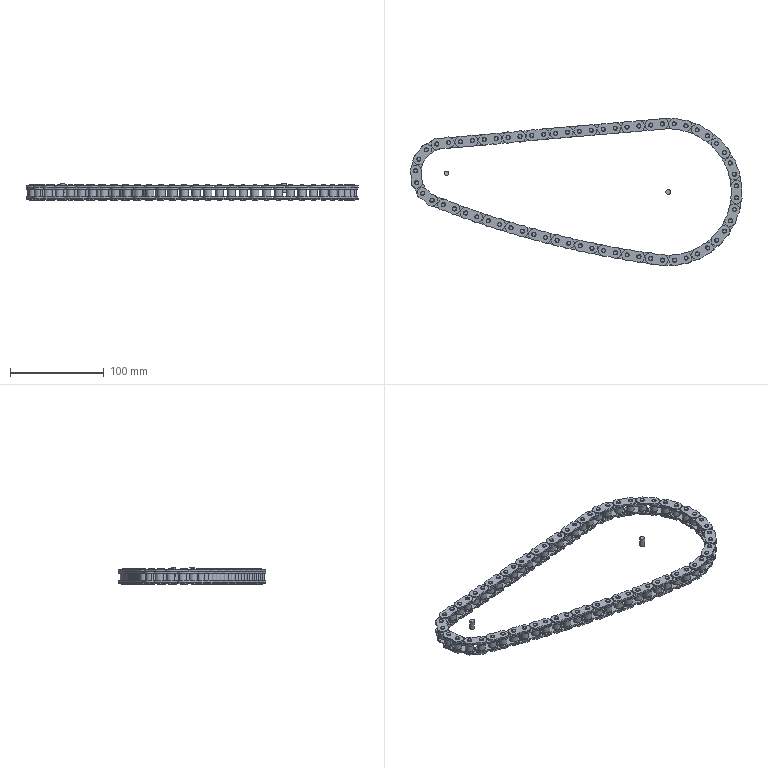Part | SolidWorks | features BaseBody 98 | 98 solids | 1928 faces | box 353.25 x 156.996 x 18.313 mm | volume 87150 mm3 | cylinder 1284 | plane 388 | cone 256 | commonest cylinder face diameters 4.45 x512 11.81 x384 57.066 x256 8.51 x128 5 x4